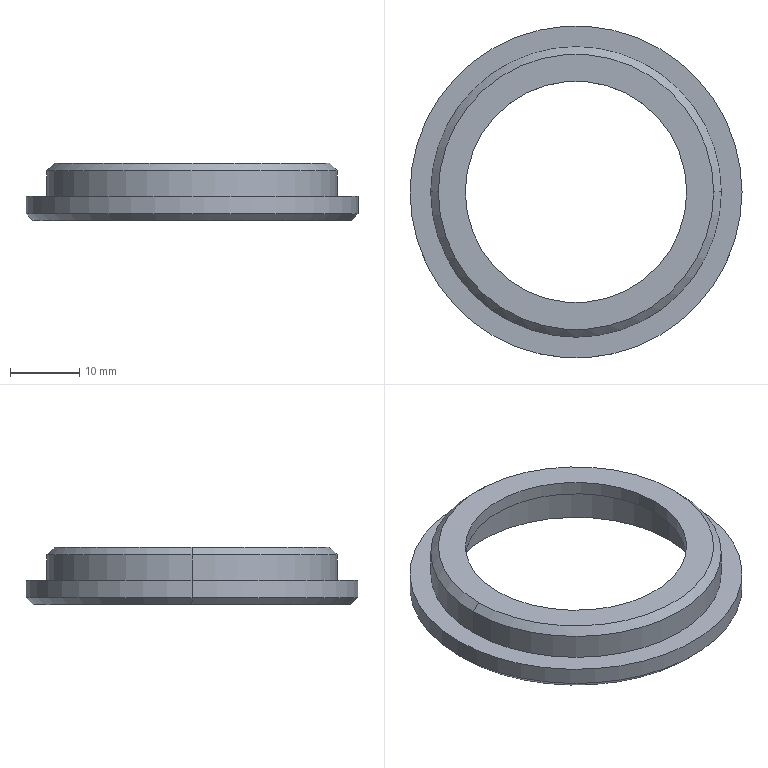Part | SolidWorks | features Chamfer 2, ICE 2, Extrusion 1 | 1 solid | 18 faces | box 48 x 48 x 8.3 mm | volume 4148 mm3 | cylinder 8 | cone 6 | plane 4 | commonest cylinder face diameters 32 x2 38 x2 42 x2 48 x2
STEP:
#1=CARTESIAN_POINT('',(-23.,0.,0.));
#2=VERTEX_POINT('',#1);
#3=CARTESIAN_POINT('',(23.,0.,0.));
#4=VERTEX_POINT('',#3);
#5=CARTESIAN_POINT('',(0.,0.,0.));
#6=DIRECTION('',(0.,0.,-1.));
#7=DIRECTION('',(1.,0.,0.));
#8=AXIS2_PLACEMENT_3D('',#5,#6,#7);
#9=CIRCLE('',#8,23.);
#10=EDGE_CURVE('',#2,#4,#9,.T.);
#11=ORIENTED_EDGE('',*,*,#10,.F.);
#12=CARTESIAN_POINT('',(-24.,0.,1.));
#13=VERTEX_POINT('',#12);
#14=CARTESIAN_POINT('',(-24.,0.,1.));
#15=DIRECTION('',(-0.7071,0.,0.7071));
#16=VECTOR('',#15,1000.);
#17=LINE('',#14,#16);
#18=EDGE_CURVE('',#2,#13,#17,.T.);
#19=ORIENTED_EDGE('',*,*,#18,.T.);
#20=CARTESIAN_POINT('',(24.,0.,1.));
#21=VERTEX_POINT('',#20);
#22=CARTESIAN_POINT('',(0.,0.,1.));
#23=DIRECTION('',(0.,0.,1.));
#24=DIRECTION('',(1.,0.,0.));
#25=AXIS2_PLACEMENT_3D('',#22,#23,#24);
#26=CIRCLE('',#25,24.);
#27=EDGE_CURVE('',#21,#13,#26,.T.);
#28=ORIENTED_EDGE('',*,*,#27,.F.);
#29=CARTESIAN_POINT('',(24.,0.,1.));
#30=DIRECTION('',(0.7071,0.,0.7071));
#31=VECTOR('',#30,1000.);
#32=LINE('',#29,#31);
#33=EDGE_CURVE('',#4,#21,#32,.T.);
#34=ORIENTED_EDGE('',*,*,#33,.F.);
#35=EDGE_LOOP('',(#11,#19,#28,#34));
#36=FACE_OUTER_BOUND('',#35,.T.);
#37=CARTESIAN_POINT('',(0.,0.,1.));
#38=DIRECTION('',(0.,0.,1.));
#39=DIRECTION('',(1.,0.,0.));
#40=AXIS2_PLACEMENT_3D('',#37,#38,#39);
#41=CONICAL_SURFACE('',#40,24.,0.7854);
#42=ADVANCED_FACE('',(#36),#41,.T.);
#43=CARTESIAN_POINT('',(19.9,0.,8.3));
#44=VERTEX_POINT('',#43);
#45=CARTESIAN_POINT('',(-19.9,0.,8.3));
#46=VERTEX_POINT('',#45);
#47=CARTESIAN_POINT('',(0.,0.,8.3));
#48=DIRECTION('',(0.,0.,1.));
#49=DIRECTION('',(1.,0.,0.));
#50=AXIS2_PLACEMENT_3D('',#47,#48,#49);
#51=CIRCLE('',#50,19.9);
#52=EDGE_CURVE('',#44,#46,#51,.T.);
#53=ORIENTED_EDGE('',*,*,#52,.F.);
#54=CARTESIAN_POINT('',(21.,0.,7.2));
#55=VERTEX_POINT('',#54);
#56=CARTESIAN_POINT('',(19.9,0.,8.3));
#57=DIRECTION('',(0.7071,0.,-0.7071));
#58=VECTOR('',#57,1000.);
#59=LINE('',#56,#58);
#60=EDGE_CURVE('',#44,#55,#59,.T.);
#61=ORIENTED_EDGE('',*,*,#60,.T.);
#62=CARTESIAN_POINT('',(-21.,0.,7.2));
#63=VERTEX_POINT('',#62);
#64=CARTESIAN_POINT('',(0.,0.,7.2));
#65=DIRECTION('',(0.,0.,-1.));
#66=DIRECTION('',(1.,0.,0.));
#67=AXIS2_PLACEMENT_3D('',#64,#65,#66);
#68=CIRCLE('',#67,21.);
#69=EDGE_CURVE('',#63,#55,#68,.T.);
#70=ORIENTED_EDGE('',*,*,#69,.F.);
#71=CARTESIAN_POINT('',(-19.9,0.,8.3));
#72=DIRECTION('',(-0.7071,0.,-0.7071));
#73=VECTOR('',#72,1000.);
#74=LINE('',#71,#73);
#75=EDGE_CURVE('',#46,#63,#74,.T.);
#76=ORIENTED_EDGE('',*,*,#75,.F.);
#77=EDGE_LOOP('',(#53,#61,#70,#76));
#78=FACE_OUTER_BOUND('',#77,.T.);
#79=CARTESIAN_POINT('',(0.,0.,8.3));
#80=DIRECTION('',(0.,0.,-1.));
#81=DIRECTION('',(-1.,0.,0.));
#82=AXIS2_PLACEMENT_3D('',#79,#80,#81);
#83=CONICAL_SURFACE('',#82,19.9,0.7854);
#84=ADVANCED_FACE('',(#78),#83,.T.);
#85=CARTESIAN_POINT('',(17.9,0.,6.3));
#86=VERTEX_POINT('',#85);
#87=CARTESIAN_POINT('',(-17.9,0.,6.3));
#88=VERTEX_POINT('',#87);
#89=CARTESIAN_POINT('',(0.,0.,6.3));
#90=DIRECTION('',(0.,0.,-1.));
#91=DIRECTION('',(1.,0.,0.));
#92=AXIS2_PLACEMENT_3D('',#89,#90,#91);
#93=CIRCLE('',#92,17.9);
#94=EDGE_CURVE('',#86,#88,#93,.T.);
#95=ORIENTED_EDGE('',*,*,#94,.F.);
#96=CARTESIAN_POINT('',(19.,0.,5.2));
#97=VERTEX_POINT('',#96);
#98=CARTESIAN_POINT('',(19.,0.,5.2));
#99=DIRECTION('',(0.7071,0.,-0.7071));
#100=VECTOR('',#99,1000.);
#101=LINE('',#98,#100);
#102=EDGE_CURVE('',#86,#97,#101,.T.);
#103=ORIENTED_EDGE('',*,*,#102,.T.);
#104=CARTESIAN_POINT('',(-19.,0.,5.2));
#105=VERTEX_POINT('',#104);
#106=CARTESIAN_POINT('',(0.,0.,5.2));
#107=DIRECTION('',(0.,0.,1.));
#108=DIRECTION('',(1.,0.,0.));
#109=AXIS2_PLACEMENT_3D('',#106,#107,#108);
#110=CIRCLE('',#109,19.);
#111=EDGE_CURVE('',#105,#97,#110,.T.);
#112=ORIENTED_EDGE('',*,*,#111,.F.);
#113=CARTESIAN_POINT('',(-19.,0.,5.2));
#114=DIRECTION('',(-0.7071,0.,-0.7071));
#115=VECTOR('',#114,1000.);
#116=LINE('',#113,#115);
#117=EDGE_CURVE('',#88,#105,#116,.T.);
#118=ORIENTED_EDGE('',*,*,#117,.F.);
#119=EDGE_LOOP('',(#95,#103,#112,#118));
#120=FACE_OUTER_BOUND('',#119,.T.);
#121=CARTESIAN_POINT('',(0.,0.,5.2));
#122=DIRECTION('',(0.,0.,-1.));
#123=DIRECTION('',(-1.,0.,0.));
#124=AXIS2_PLACEMENT_3D('',#121,#122,#123);
#125=CONICAL_SURFACE('',#124,19.,0.7854);
#126=ADVANCED_FACE('',(#120),#125,.F.);
#127=CARTESIAN_POINT('',(-16.,0.,8.3));
#128=VERTEX_POINT('',#127);
#129=CARTESIAN_POINT('',(16.,0.,8.3));
#130=VERTEX_POINT('',#129);
#131=CARTESIAN_POINT('',(0.,0.,8.3));
#132=DIRECTION('',(0.,0.,1.));
#133=DIRECTION('',(1.,0.,0.));
#134=AXIS2_PLACEMENT_3D('',#131,#132,#133);
#135=CIRCLE('',#134,16.);
#136=EDGE_CURVE('',#128,#130,#135,.T.);
#137=ORIENTED_EDGE('',*,*,#136,.T.);
#138=CARTESIAN_POINT('',(16.,0.,6.3));
#139=VERTEX_POINT('',#138);
#140=CARTESIAN_POINT('',(16.,0.,8.3));
#141=DIRECTION('',(0.,0.,-1.));
#142=VECTOR('',#141,1000.);
#143=LINE('',#140,#142);
#144=EDGE_CURVE('',#130,#139,#143,.T.);
#145=ORIENTED_EDGE('',*,*,#144,.T.);
#146=CARTESIAN_POINT('',(-16.,0.,6.3));
#147=VERTEX_POINT('',#146);
#148=CARTESIAN_POINT('',(0.,0.,6.3));
#149=DIRECTION('',(0.,0.,1.));
#150=DIRECTION('',(1.,0.,0.));
#151=AXIS2_PLACEMENT_3D('',#148,#149,#150);
#152=CIRCLE('',#151,16.);
#153=EDGE_CURVE('',#147,#139,#152,.T.);
#154=ORIENTED_EDGE('',*,*,#153,.F.);
#155=CARTESIAN_POINT('',(-16.,0.,8.3));
#156=DIRECTION('',(0.,0.,-1.));
#157=VECTOR('',#156,1000.);
#158=LINE('',#155,#157);
#159=EDGE_CURVE('',#128,#147,#158,.T.);
#160=ORIENTED_EDGE('',*,*,#159,.F.);
#161=EDGE_LOOP('',(#137,#145,#154,#160));
#162=FACE_OUTER_BOUND('',#161,.T.);
#163=CARTESIAN_POINT('',(0.,0.,8.3));
#164=DIRECTION('',(0.,0.,-1.));
#165=DIRECTION('',(-1.,0.,0.));
#166=AXIS2_PLACEMENT_3D('',#163,#164,#165);
#167=CYLINDRICAL_SURFACE('',#166,16.);
#168=ADVANCED_FACE('',(#162),#167,.F.);
#169=ORIENTED_EDGE('',*,*,#69,.T.);
#170=CARTESIAN_POINT('',(21.,0.,3.5));
#171=VERTEX_POINT('',#170);
#172=CARTESIAN_POINT('',(21.,0.,6.3));
#173=DIRECTION('',(0.,0.,-1.));
#174=VECTOR('',#173,1000.);
#175=LINE('',#172,#174);
#176=EDGE_CURVE('',#55,#171,#175,.T.);
#177=ORIENTED_EDGE('',*,*,#176,.T.);
#178=CARTESIAN_POINT('',(-21.,0.,3.5));
#179=VERTEX_POINT('',#178);
#180=CARTESIAN_POINT('',(0.,0.,3.5));
#181=DIRECTION('',(0.,0.,1.));
#182=DIRECTION('',(1.,0.,0.));
#183=AXIS2_PLACEMENT_3D('',#180,#181,#182);
#184=CIRCLE('',#183,21.);
#185=EDGE_CURVE('',#171,#179,#184,.T.);
#186=ORIENTED_EDGE('',*,*,#185,.T.);
#187=CARTESIAN_POINT('',(-21.,0.,6.3));
#188=DIRECTION('',(0.,0.,-1.));
#189=VECTOR('',#188,1000.);
#190=LINE('',#187,#189);
#191=EDGE_CURVE('',#63,#179,#190,.T.);
#192=ORIENTED_EDGE('',*,*,#191,.F.);
#193=EDGE_LOOP('',(#169,#177,#186,#192));
#194=FACE_OUTER_BOUND('',#193,.T.);
#195=CARTESIAN_POINT('',(0.,0.,6.3));
#196=DIRECTION('',(0.,0.,-1.));
#197=DIRECTION('',(-1.,0.,0.));
#198=AXIS2_PLACEMENT_3D('',#195,#196,#197);
#199=CYLINDRICAL_SURFACE('',#198,21.);
#200=ADVANCED_FACE('',(#194),#199,.T.);
#201=ORIENTED_EDGE('',*,*,#111,.T.);
#202=CARTESIAN_POINT('',(19.,0.,0.));
#203=VERTEX_POINT('',#202);
#204=CARTESIAN_POINT('',(19.,0.,3.5));
#205=DIRECTION('',(0.,0.,-1.));
#206=VECTOR('',#205,1000.);
#207=LINE('',#204,#206);
#208=EDGE_CURVE('',#97,#203,#207,.T.);
#209=ORIENTED_EDGE('',*,*,#208,.T.);
#210=CARTESIAN_POINT('',(-19.,0.,0.));
#211=VERTEX_POINT('',#210);
#212=CARTESIAN_POINT('',(0.,0.,0.));
#213=DIRECTION('',(0.,0.,1.));
#214=DIRECTION('',(1.,0.,0.));
#215=AXIS2_PLACEMENT_3D('',#212,#213,#214);
#216=CIRCLE('',#215,19.);
#217=EDGE_CURVE('',#211,#203,#216,.T.);
#218=ORIENTED_EDGE('',*,*,#217,.F.);
#219=CARTESIAN_POINT('',(-19.,0.,3.5));
#220=DIRECTION('',(0.,0.,-1.));
#221=VECTOR('',#220,1000.);
#222=LINE('',#219,#221);
#223=EDGE_CURVE('',#105,#211,#222,.T.);
#224=ORIENTED_EDGE('',*,*,#223,.F.);
#225=EDGE_LOOP('',(#201,#209,#218,#224));
#226=FACE_OUTER_BOUND('',#225,.T.);
#227=CARTESIAN_POINT('',(0.,0.,3.5));
#228=DIRECTION('',(0.,0.,-1.));
#229=DIRECTION('',(-1.,0.,0.));
#230=AXIS2_PLACEMENT_3D('',#227,#228,#229);
#231=CYLINDRICAL_SURFACE('',#230,19.);
#232=ADVANCED_FACE('',(#226),#231,.F.);
#233=CARTESIAN_POINT('',(24.,0.,3.5));
#234=VERTEX_POINT('',#233);
#235=CARTESIAN_POINT('',(-24.,0.,3.5));
#236=VERTEX_POINT('',#235);
#237=CARTESIAN_POINT('',(0.,0.,3.5));
#238=DIRECTION('',(0.,0.,1.));
#239=DIRECTION('',(1.,0.,0.));
#240=AXIS2_PLACEMENT_3D('',#237,#238,#239);
#241=CIRCLE('',#240,24.);
#242=EDGE_CURVE('',#234,#236,#241,.T.);
#243=ORIENTED_EDGE('',*,*,#242,.F.);
#244=CARTESIAN_POINT('',(24.,0.,3.5));
#245=DIRECTION('',(0.,0.,-1.));
#246=VECTOR('',#245,1000.);
#247=LINE('',#244,#246);
#248=EDGE_CURVE('',#234,#21,#247,.T.);
#249=ORIENTED_EDGE('',*,*,#248,.T.);
#250=ORIENTED_EDGE('',*,*,#27,.T.);
#251=CARTESIAN_POINT('',(-24.,0.,3.5));
#252=DIRECTION('',(0.,0.,-1.));
#253=VECTOR('',#252,1000.);
#254=LINE('',#251,#253);
#255=EDGE_CURVE('',#236,#13,#254,.T.);
#256=ORIENTED_EDGE('',*,*,#255,.F.);
#257=EDGE_LOOP('',(#243,#249,#250,#256));
#258=FACE_OUTER_BOUND('',#257,.T.);
#259=CARTESIAN_POINT('',(0.,0.,3.5));
#260=DIRECTION('',(0.,0.,-1.));
#261=DIRECTION('',(-1.,0.,0.));
#262=AXIS2_PLACEMENT_3D('',#259,#260,#261);
#263=CYLINDRICAL_SURFACE('',#262,24.);
#264=ADVANCED_FACE('',(#258),#263,.T.);
#265=CARTESIAN_POINT('',(0.,0.,3.5));
#266=DIRECTION('',(0.,0.,1.));
#267=DIRECTION('',(1.,0.,0.));
#268=AXIS2_PLACEMENT_3D('',#265,#266,#267);
#269=CIRCLE('',#268,24.);
#270=EDGE_CURVE('',#236,#234,#269,.T.);
#271=ORIENTED_EDGE('',*,*,#270,.T.);
#272=ORIENTED_EDGE('',*,*,#242,.T.);
#273=EDGE_LOOP('',(#271,#272));
#274=FACE_OUTER_BOUND('',#273,.T.);
#275=CARTESIAN_POINT('',(0.,0.,3.5));
#276=DIRECTION('',(0.,0.,1.));
#277=DIRECTION('',(1.,0.,0.));
#278=AXIS2_PLACEMENT_3D('',#275,#276,#277);
#279=CIRCLE('',#278,21.);
#280=EDGE_CURVE('',#179,#171,#279,.T.);
#281=ORIENTED_EDGE('',*,*,#280,.F.);
#282=ORIENTED_EDGE('',*,*,#185,.F.);
#283=EDGE_LOOP('',(#281,#282));
#284=FACE_BOUND('',#283,.T.);
#285=CARTESIAN_POINT('',(0.,0.,3.5));
#286=DIRECTION('',(0.,0.,1.));
#287=DIRECTION('',(1.,0.,0.));
#288=AXIS2_PLACEMENT_3D('',#285,#286,#287);
#289=PLANE('',#288);
#290=ADVANCED_FACE('',(#274,#284),#289,.T.);
#291=CARTESIAN_POINT('',(0.,0.,0.));
#292=DIRECTION('',(0.,0.,-1.));
#293=DIRECTION('',(1.,0.,0.));
#294=AXIS2_PLACEMENT_3D('',#291,#292,#293);
#295=CIRCLE('',#294,23.);
#296=EDGE_CURVE('',#4,#2,#295,.T.);
#297=ORIENTED_EDGE('',*,*,#296,.T.);
#298=ORIENTED_EDGE('',*,*,#10,.T.);
#299=EDGE_LOOP('',(#297,#298));
#300=FACE_OUTER_BOUND('',#299,.T.);
#301=ORIENTED_EDGE('',*,*,#217,.T.);
#302=CARTESIAN_POINT('',(0.,0.,0.));
#303=DIRECTION('',(0.,0.,1.));
#304=DIRECTION('',(1.,0.,0.));
#305=AXIS2_PLACEMENT_3D('',#302,#303,#304);
#306=CIRCLE('',#305,19.);
#307=EDGE_CURVE('',#203,#211,#306,.T.);
#308=ORIENTED_EDGE('',*,*,#307,.T.);
#309=EDGE_LOOP('',(#301,#308));
#310=FACE_BOUND('',#309,.T.);
#311=CARTESIAN_POINT('',(0.,0.,0.));
#312=DIRECTION('',(0.,0.,1.));
#313=DIRECTION('',(1.,0.,0.));
#314=AXIS2_PLACEMENT_3D('',#311,#312,#313);
#315=PLANE('',#314);
#316=ADVANCED_FACE('',(#300,#310),#315,.F.);
#317=ORIENTED_EDGE('',*,*,#248,.F.);
#318=ORIENTED_EDGE('',*,*,#270,.F.);
#319=ORIENTED_EDGE('',*,*,#255,.T.);
#320=CARTESIAN_POINT('',(0.,0.,1.));
#321=DIRECTION('',(0.,0.,1.));
#322=DIRECTION('',(1.,0.,0.));
#323=AXIS2_PLACEMENT_3D('',#320,#321,#322);
#324=CIRCLE('',#323,24.);
#325=EDGE_CURVE('',#13,#21,#324,.T.);
#326=ORIENTED_EDGE('',*,*,#325,.T.);
#327=EDGE_LOOP('',(#317,#318,#319,#326));
#328=FACE_OUTER_BOUND('',#327,.T.);
#329=CARTESIAN_POINT('',(0.,0.,3.5));
#330=DIRECTION('',(0.,0.,-1.));
#331=DIRECTION('',(-1.,0.,0.));
#332=AXIS2_PLACEMENT_3D('',#329,#330,#331);
#333=CYLINDRICAL_SURFACE('',#332,24.);
#334=ADVANCED_FACE('',(#328),#333,.T.);
#335=ORIENTED_EDGE('',*,*,#208,.F.);
#336=CARTESIAN_POINT('',(0.,0.,5.2));
#337=DIRECTION('',(0.,0.,1.));
#338=DIRECTION('',(1.,0.,0.));
#339=AXIS2_PLACEMENT_3D('',#336,#337,#338);
#340=CIRCLE('',#339,19.);
#341=EDGE_CURVE('',#97,#105,#340,.T.);
#342=ORIENTED_EDGE('',*,*,#341,.T.);
#343=ORIENTED_EDGE('',*,*,#223,.T.);
#344=ORIENTED_EDGE('',*,*,#307,.F.);
#345=EDGE_LOOP('',(#335,#342,#343,#344));
#346=FACE_OUTER_BOUND('',#345,.T.);
#347=CARTESIAN_POINT('',(0.,0.,3.5));
#348=DIRECTION('',(0.,0.,-1.));
#349=DIRECTION('',(-1.,0.,0.));
#350=AXIS2_PLACEMENT_3D('',#347,#348,#349);
#351=CYLINDRICAL_SURFACE('',#350,19.);
#352=ADVANCED_FACE('',(#346),#351,.F.);
#353=ORIENTED_EDGE('',*,*,#176,.F.);
#354=CARTESIAN_POINT('',(0.,0.,7.2));
#355=DIRECTION('',(0.,0.,-1.));
#356=DIRECTION('',(1.,0.,0.));
#357=AXIS2_PLACEMENT_3D('',#354,#355,#356);
#358=CIRCLE('',#357,21.);
#359=EDGE_CURVE('',#55,#63,#358,.T.);
#360=ORIENTED_EDGE('',*,*,#359,.T.);
#361=ORIENTED_EDGE('',*,*,#191,.T.);
#362=ORIENTED_EDGE('',*,*,#280,.T.);
#363=EDGE_LOOP('',(#353,#360,#361,#362));
#364=FACE_OUTER_BOUND('',#363,.T.);
#365=CARTESIAN_POINT('',(0.,0.,6.3));
#366=DIRECTION('',(0.,0.,-1.));
#367=DIRECTION('',(-1.,0.,0.));
#368=AXIS2_PLACEMENT_3D('',#365,#366,#367);
#369=CYLINDRICAL_SURFACE('',#368,21.);
#370=ADVANCED_FACE('',(#364),#369,.T.);
#371=CARTESIAN_POINT('',(0.,0.,6.3));
#372=DIRECTION('',(0.,0.,-1.));
#373=DIRECTION('',(1.,0.,0.));
#374=AXIS2_PLACEMENT_3D('',#371,#372,#373);
#375=CIRCLE('',#374,17.9);
#376=EDGE_CURVE('',#88,#86,#375,.T.);
#377=ORIENTED_EDGE('',*,*,#376,.T.);
#378=ORIENTED_EDGE('',*,*,#94,.T.);
#379=EDGE_LOOP('',(#377,#378));
#380=FACE_OUTER_BOUND('',#379,.T.);
#381=ORIENTED_EDGE('',*,*,#153,.T.);
#382=CARTESIAN_POINT('',(0.,0.,6.3));
#383=DIRECTION('',(0.,0.,1.));
#384=DIRECTION('',(1.,0.,0.));
#385=AXIS2_PLACEMENT_3D('',#382,#383,#384);
#386=CIRCLE('',#385,16.);
#387=EDGE_CURVE('',#139,#147,#386,.T.);
#388=ORIENTED_EDGE('',*,*,#387,.T.);
#389=EDGE_LOOP('',(#381,#388));
#390=FACE_BOUND('',#389,.T.);
#391=CARTESIAN_POINT('',(0.,0.,6.3));
#392=DIRECTION('',(0.,0.,1.));
#393=DIRECTION('',(1.,0.,0.));
#394=AXIS2_PLACEMENT_3D('',#391,#392,#393);
#395=PLANE('',#394);
#396=ADVANCED_FACE('',(#380,#390),#395,.F.);
#397=CARTESIAN_POINT('',(0.,0.,8.3));
#398=DIRECTION('',(0.,0.,1.));
#399=DIRECTION('',(1.,0.,0.));
#400=AXIS2_PLACEMENT_3D('',#397,#398,#399);
#401=CIRCLE('',#400,19.9);
#402=EDGE_CURVE('',#46,#44,#401,.T.);
#403=ORIENTED_EDGE('',*,*,#402,.T.);
#404=ORIENTED_EDGE('',*,*,#52,.T.);
#405=EDGE_LOOP('',(#403,#404));
#406=FACE_OUTER_BOUND('',#405,.T.);
#407=ORIENTED_EDGE('',*,*,#136,.F.);
#408=CARTESIAN_POINT('',(0.,0.,8.3));
#409=DIRECTION('',(0.,0.,1.));
#410=DIRECTION('',(1.,0.,0.));
#411=AXIS2_PLACEMENT_3D('',#408,#409,#410);
#412=CIRCLE('',#411,16.);
#413=EDGE_CURVE('',#130,#128,#412,.T.);
#414=ORIENTED_EDGE('',*,*,#413,.F.);
#415=EDGE_LOOP('',(#407,#414));
#416=FACE_BOUND('',#415,.T.);
#417=CARTESIAN_POINT('',(0.,0.,8.3));
#418=DIRECTION('',(0.,0.,1.));
#419=DIRECTION('',(1.,0.,0.));
#420=AXIS2_PLACEMENT_3D('',#417,#418,#419);
#421=PLANE('',#420);
#422=ADVANCED_FACE('',(#406,#416),#421,.T.);
#423=ORIENTED_EDGE('',*,*,#144,.F.);
#424=ORIENTED_EDGE('',*,*,#413,.T.);
#425=ORIENTED_EDGE('',*,*,#159,.T.);
#426=ORIENTED_EDGE('',*,*,#387,.F.);
#427=EDGE_LOOP('',(#423,#424,#425,#426));
#428=FACE_OUTER_BOUND('',#427,.T.);
#429=CARTESIAN_POINT('',(0.,0.,8.3));
#430=DIRECTION('',(0.,0.,-1.));
#431=DIRECTION('',(-1.,0.,0.));
#432=AXIS2_PLACEMENT_3D('',#429,#430,#431);
#433=CYLINDRICAL_SURFACE('',#432,16.);
#434=ADVANCED_FACE('',(#428),#433,.F.);
#435=ORIENTED_EDGE('',*,*,#102,.F.);
#436=ORIENTED_EDGE('',*,*,#376,.F.);
#437=ORIENTED_EDGE('',*,*,#117,.T.);
#438=ORIENTED_EDGE('',*,*,#341,.F.);
#439=EDGE_LOOP('',(#435,#436,#437,#438));
#440=FACE_OUTER_BOUND('',#439,.T.);
#441=CARTESIAN_POINT('',(0.,0.,5.2));
#442=DIRECTION('',(0.,0.,-1.));
#443=DIRECTION('',(-1.,0.,0.));
#444=AXIS2_PLACEMENT_3D('',#441,#442,#443);
#445=CONICAL_SURFACE('',#444,19.,0.7854);
#446=ADVANCED_FACE('',(#440),#445,.F.);
#447=ORIENTED_EDGE('',*,*,#60,.F.);
#448=ORIENTED_EDGE('',*,*,#402,.F.);
#449=ORIENTED_EDGE('',*,*,#75,.T.);
#450=ORIENTED_EDGE('',*,*,#359,.F.);
#451=EDGE_LOOP('',(#447,#448,#449,#450));
#452=FACE_OUTER_BOUND('',#451,.T.);
#453=CARTESIAN_POINT('',(0.,0.,8.3));
#454=DIRECTION('',(0.,0.,-1.));
#455=DIRECTION('',(-1.,0.,0.));
#456=AXIS2_PLACEMENT_3D('',#453,#454,#455);
#457=CONICAL_SURFACE('',#456,19.9,0.7854);
#458=ADVANCED_FACE('',(#452),#457,.T.);
#459=ORIENTED_EDGE('',*,*,#18,.F.);
#460=ORIENTED_EDGE('',*,*,#296,.F.);
#461=ORIENTED_EDGE('',*,*,#33,.T.);
#462=ORIENTED_EDGE('',*,*,#325,.F.);
#463=EDGE_LOOP('',(#459,#460,#461,#462));
#464=FACE_OUTER_BOUND('',#463,.T.);
#465=CARTESIAN_POINT('',(0.,0.,1.));
#466=DIRECTION('',(0.,0.,1.));
#467=DIRECTION('',(1.,0.,0.));
#468=AXIS2_PLACEMENT_3D('',#465,#466,#467);
#469=CONICAL_SURFACE('',#468,24.,0.7854);
#470=ADVANCED_FACE('',(#464),#469,.T.);
#471=CLOSED_SHELL('',(#42,#84,#126,#168,#200,#232,#264,#290,#316,#334,#352,#370,#396,#422,#434,#446,#458,#470));
#472=MANIFOLD_SOLID_BREP('',#471);
#473=CARTESIAN_POINT('',(0.,0.,0.));
#474=DIRECTION('',(0.,0.,1.));
#475=DIRECTION('',(1.,0.,0.));
#476=AXIS2_PLACEMENT_3D('',#473,#474,#475);
#477=(LENGTH_UNIT()NAMED_UNIT(*)SI_UNIT(.MILLI.,.METRE.));
#478=UNCERTAINTY_MEASURE_WITH_UNIT(LENGTH_MEASURE(0.00001),#477,'','');
#479=(NAMED_UNIT(*)PLANE_ANGLE_UNIT()SI_UNIT($,.RADIAN.));
#480=(NAMED_UNIT(*)SI_UNIT($,.STERADIAN.)SOLID_ANGLE_UNIT());
#481=(GEOMETRIC_REPRESENTATION_CONTEXT(3)GLOBAL_UNCERTAINTY_ASSIGNED_CONTEXT((#478))GLOBAL_UNIT_ASSIGNED_CONTEXT((#477,#479,#480))REPRESENTATION_CONTEXT('',''));
#482=ADVANCED_BREP_SHAPE_REPRESENTATION('',(#472,#476),#481);